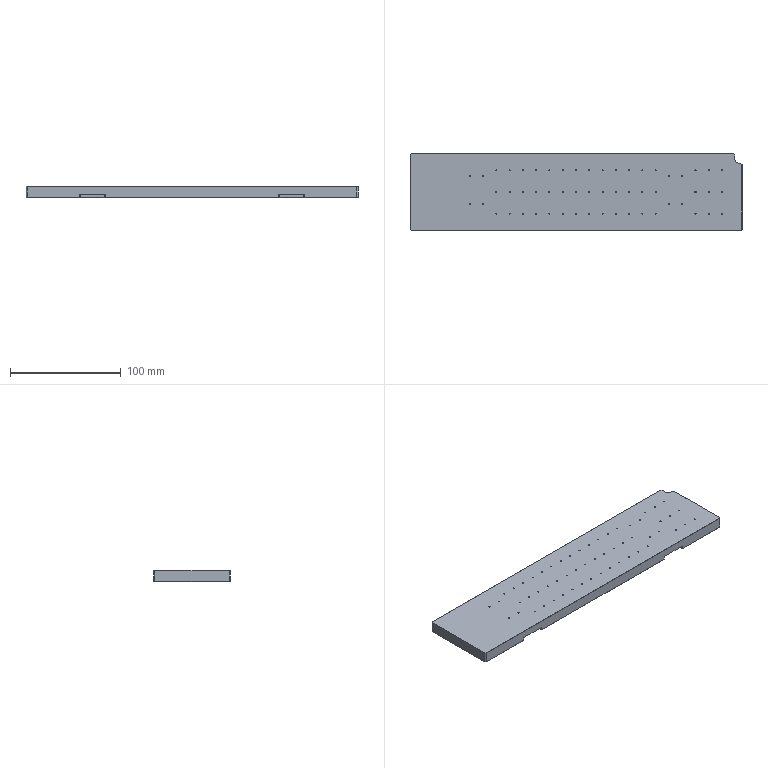Part | NX | features BREP 1 | 1 solid | 475 faces | box 300 x 69 x 10 mm | volume 185896 mm3 | cylinder 307 | plane 86 | cone 82 | commonest cylinder face diameters 4 x172 1 x112 2 x8 2.5 x8 4.2 x6 8 x1